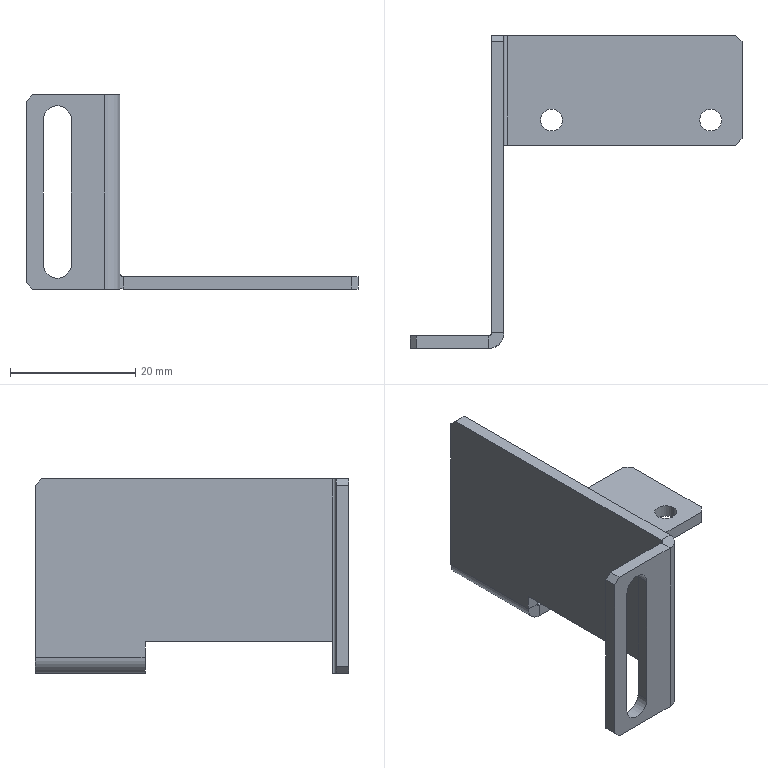Part | STEP file | 11-GX-ZB-04-006-A11 | 1 solid | 39 faces | box 53 x 50 x 31 mm | volume 4591 mm3 | plane 29 | cylinder 10 | commonest cylinder face diameters 3.5 x4 1 x2 4.5 x2 5 x2
STEP:
#1=CARTESIAN_POINT('',(34.75,-13.5,0.));
#2=VERTEX_POINT('',#1);
#3=CARTESIAN_POINT('',(31.25,-13.5,0.));
#4=VERTEX_POINT('',#3);
#5=CARTESIAN_POINT('',(33.,-13.5,0.));
#6=DIRECTION('',(0.,0.,-1.));
#7=DIRECTION('',(-1.,0.,0.));
#8=AXIS2_PLACEMENT_3D('',#5,#6,#7);
#9=CIRCLE('',#8,1.75);
#10=EDGE_CURVE('',#2,#4,#9,.T.);
#11=ORIENTED_EDGE('',*,*,#10,.T.);
#12=CARTESIAN_POINT('',(31.25,-13.5,2.));
#13=VERTEX_POINT('',#12);
#14=CARTESIAN_POINT('',(31.25,-13.5,-8.));
#15=DIRECTION('',(0.,0.,1.));
#16=VECTOR('',#15,1000.);
#17=LINE('',#14,#16);
#18=EDGE_CURVE('',#4,#13,#17,.T.);
#19=ORIENTED_EDGE('',*,*,#18,.T.);
#20=CARTESIAN_POINT('',(34.75,-13.5,2.));
#21=VERTEX_POINT('',#20);
#22=CARTESIAN_POINT('',(33.,-13.5,2.));
#23=DIRECTION('',(0.,0.,1.));
#24=DIRECTION('',(1.,0.,0.));
#25=AXIS2_PLACEMENT_3D('',#22,#23,#24);
#26=CIRCLE('',#25,1.75);
#27=EDGE_CURVE('',#13,#21,#26,.T.);
#28=ORIENTED_EDGE('',*,*,#27,.T.);
#29=CARTESIAN_POINT('',(34.75,-13.5,-8.));
#30=DIRECTION('',(0.,0.,1.));
#31=VECTOR('',#30,1000.);
#32=LINE('',#29,#31);
#33=EDGE_CURVE('',#2,#21,#32,.T.);
#34=ORIENTED_EDGE('',*,*,#33,.F.);
#35=EDGE_LOOP('',(#11,#19,#28,#34));
#36=FACE_OUTER_BOUND('',#35,.T.);
#37=CARTESIAN_POINT('',(33.,-13.5,-8.));
#38=DIRECTION('',(0.,0.,1.));
#39=DIRECTION('',(1.,0.,0.));
#40=AXIS2_PLACEMENT_3D('',#37,#38,#39);
#41=CYLINDRICAL_SURFACE('',#40,1.75);
#42=ADVANCED_FACE('',(#36),#41,.F.);
#43=CARTESIAN_POINT('',(9.35,-13.5,0.));
#44=VERTEX_POINT('',#43);
#45=CARTESIAN_POINT('',(5.85,-13.5,0.));
#46=VERTEX_POINT('',#45);
#47=CARTESIAN_POINT('',(7.6,-13.5,0.));
#48=DIRECTION('',(0.,0.,-1.));
#49=DIRECTION('',(-1.,0.,0.));
#50=AXIS2_PLACEMENT_3D('',#47,#48,#49);
#51=CIRCLE('',#50,1.75);
#52=EDGE_CURVE('',#44,#46,#51,.T.);
#53=ORIENTED_EDGE('',*,*,#52,.T.);
#54=CARTESIAN_POINT('',(5.85,-13.5,2.));
#55=VERTEX_POINT('',#54);
#56=CARTESIAN_POINT('',(5.85,-13.5,-8.));
#57=DIRECTION('',(0.,0.,1.));
#58=VECTOR('',#57,1000.);
#59=LINE('',#56,#58);
#60=EDGE_CURVE('',#46,#55,#59,.T.);
#61=ORIENTED_EDGE('',*,*,#60,.T.);
#62=CARTESIAN_POINT('',(9.35,-13.5,2.));
#63=VERTEX_POINT('',#62);
#64=CARTESIAN_POINT('',(7.6,-13.5,2.));
#65=DIRECTION('',(0.,0.,1.));
#66=DIRECTION('',(1.,0.,0.));
#67=AXIS2_PLACEMENT_3D('',#64,#65,#66);
#68=CIRCLE('',#67,1.75);
#69=EDGE_CURVE('',#55,#63,#68,.T.);
#70=ORIENTED_EDGE('',*,*,#69,.T.);
#71=CARTESIAN_POINT('',(9.35,-13.5,-8.));
#72=DIRECTION('',(0.,0.,1.));
#73=VECTOR('',#72,1000.);
#74=LINE('',#71,#73);
#75=EDGE_CURVE('',#44,#63,#74,.T.);
#76=ORIENTED_EDGE('',*,*,#75,.F.);
#77=EDGE_LOOP('',(#53,#61,#70,#76));
#78=FACE_OUTER_BOUND('',#77,.T.);
#79=CARTESIAN_POINT('',(7.6,-13.5,-8.));
#80=DIRECTION('',(0.,0.,1.));
#81=DIRECTION('',(1.,0.,0.));
#82=AXIS2_PLACEMENT_3D('',#79,#80,#81);
#83=CYLINDRICAL_SURFACE('',#82,1.75);
#84=ADVANCED_FACE('',(#78),#83,.F.);
#85=CARTESIAN_POINT('',(-2.,-1.,31.));
#86=VERTEX_POINT('',#85);
#87=CARTESIAN_POINT('',(-2.,-47.5,31.));
#88=VERTEX_POINT('',#87);
#89=CARTESIAN_POINT('',(-2.,0.,31.));
#90=DIRECTION('',(0.,-1.,0.));
#91=VECTOR('',#90,1000.);
#92=LINE('',#89,#91);
#93=EDGE_CURVE('',#86,#88,#92,.T.);
#94=ORIENTED_EDGE('',*,*,#93,.F.);
#95=CARTESIAN_POINT('',(-2.,0.,30.));
#96=VERTEX_POINT('',#95);
#97=CARTESIAN_POINT('',(-2.,0.,30.));
#98=DIRECTION('',(0.,0.7071,-0.7071));
#99=VECTOR('',#98,1000.);
#100=LINE('',#97,#99);
#101=EDGE_CURVE('',#86,#96,#100,.T.);
#102=ORIENTED_EDGE('',*,*,#101,.T.);
#103=CARTESIAN_POINT('',(-2.,0.,2.5));
#104=VERTEX_POINT('',#103);
#105=CARTESIAN_POINT('',(-2.,0.,31.));
#106=DIRECTION('',(0.,0.,-1.));
#107=VECTOR('',#106,1000.);
#108=LINE('',#105,#107);
#109=EDGE_CURVE('',#96,#104,#108,.T.);
#110=ORIENTED_EDGE('',*,*,#109,.T.);
#111=CARTESIAN_POINT('',(-2.,-17.5,2.5));
#112=VERTEX_POINT('',#111);
#113=CARTESIAN_POINT('',(-2.,0.,2.5));
#114=DIRECTION('',(0.,-1.,0.));
#115=VECTOR('',#114,1000.);
#116=LINE('',#113,#115);
#117=EDGE_CURVE('',#104,#112,#116,.T.);
#118=ORIENTED_EDGE('',*,*,#117,.T.);
#119=CARTESIAN_POINT('',(-2.,-17.5,5.));
#120=VERTEX_POINT('',#119);
#121=CARTESIAN_POINT('',(-2.,-17.5,31.));
#122=DIRECTION('',(0.,0.,1.));
#123=VECTOR('',#122,1000.);
#124=LINE('',#121,#123);
#125=EDGE_CURVE('',#112,#120,#124,.T.);
#126=ORIENTED_EDGE('',*,*,#125,.T.);
#127=CARTESIAN_POINT('',(-2.,-47.5,5.));
#128=VERTEX_POINT('',#127);
#129=CARTESIAN_POINT('',(-2.,0.,5.));
#130=DIRECTION('',(0.,-1.,0.));
#131=VECTOR('',#130,1000.);
#132=LINE('',#129,#131);
#133=EDGE_CURVE('',#120,#128,#132,.T.);
#134=ORIENTED_EDGE('',*,*,#133,.T.);
#135=CARTESIAN_POINT('',(-2.,-47.5,31.));
#136=DIRECTION('',(0.,0.,-1.));
#137=VECTOR('',#136,1000.);
#138=LINE('',#135,#137);
#139=EDGE_CURVE('',#88,#128,#138,.T.);
#140=ORIENTED_EDGE('',*,*,#139,.F.);
#141=EDGE_LOOP('',(#94,#102,#110,#118,#126,#134,#140));
#142=FACE_OUTER_BOUND('',#141,.T.);
#143=CARTESIAN_POINT('',(-2.,0.,31.));
#144=DIRECTION('',(1.,0.,0.));
#145=DIRECTION('',(0.,1.,0.));
#146=AXIS2_PLACEMENT_3D('',#143,#144,#145);
#147=PLANE('',#146);
#148=ADVANCED_FACE('',(#142),#147,.F.);
#149=CARTESIAN_POINT('',(0.,0.,30.));
#150=VERTEX_POINT('',#149);
#151=CARTESIAN_POINT('',(0.,0.,2.5));
#152=VERTEX_POINT('',#151);
#153=CARTESIAN_POINT('',(0.,0.,31.));
#154=DIRECTION('',(0.,0.,-1.));
#155=VECTOR('',#154,1000.);
#156=LINE('',#153,#155);
#157=EDGE_CURVE('',#150,#152,#156,.T.);
#158=ORIENTED_EDGE('',*,*,#157,.F.);
#159=CARTESIAN_POINT('',(0.,-1.,31.));
#160=VERTEX_POINT('',#159);
#161=CARTESIAN_POINT('',(0.,-0.5,30.5));
#162=DIRECTION('',(0.,-0.7071,0.7071));
#163=VECTOR('',#162,1000.);
#164=LINE('',#161,#163);
#165=EDGE_CURVE('',#150,#160,#164,.T.);
#166=ORIENTED_EDGE('',*,*,#165,.T.);
#167=CARTESIAN_POINT('',(0.,-47.5,31.));
#168=VERTEX_POINT('',#167);
#169=CARTESIAN_POINT('',(0.,0.,31.));
#170=DIRECTION('',(0.,-1.,0.));
#171=VECTOR('',#170,1000.);
#172=LINE('',#169,#171);
#173=EDGE_CURVE('',#160,#168,#172,.T.);
#174=ORIENTED_EDGE('',*,*,#173,.T.);
#175=CARTESIAN_POINT('',(0.,-47.5,5.));
#176=VERTEX_POINT('',#175);
#177=CARTESIAN_POINT('',(0.,-47.5,31.));
#178=DIRECTION('',(0.,0.,-1.));
#179=VECTOR('',#178,1000.);
#180=LINE('',#177,#179);
#181=EDGE_CURVE('',#168,#176,#180,.T.);
#182=ORIENTED_EDGE('',*,*,#181,.T.);
#183=CARTESIAN_POINT('',(0.,-17.5,5.));
#184=VERTEX_POINT('',#183);
#185=CARTESIAN_POINT('',(0.,0.,5.));
#186=DIRECTION('',(0.,-1.,0.));
#187=VECTOR('',#186,1000.);
#188=LINE('',#185,#187);
#189=EDGE_CURVE('',#184,#176,#188,.T.);
#190=ORIENTED_EDGE('',*,*,#189,.F.);
#191=CARTESIAN_POINT('',(0.,-17.5,2.5));
#192=VERTEX_POINT('',#191);
#193=CARTESIAN_POINT('',(0.,-17.5,31.));
#194=DIRECTION('',(0.,0.,1.));
#195=VECTOR('',#194,1000.);
#196=LINE('',#193,#195);
#197=EDGE_CURVE('',#192,#184,#196,.T.);
#198=ORIENTED_EDGE('',*,*,#197,.F.);
#199=CARTESIAN_POINT('',(0.,0.,2.5));
#200=DIRECTION('',(0.,-1.,0.));
#201=VECTOR('',#200,1000.);
#202=LINE('',#199,#201);
#203=EDGE_CURVE('',#152,#192,#202,.T.);
#204=ORIENTED_EDGE('',*,*,#203,.F.);
#205=EDGE_LOOP('',(#158,#166,#174,#182,#190,#198,#204));
#206=FACE_OUTER_BOUND('',#205,.T.);
#207=CARTESIAN_POINT('',(0.,0.,31.));
#208=DIRECTION('',(1.,0.,0.));
#209=DIRECTION('',(0.,1.,0.));
#210=AXIS2_PLACEMENT_3D('',#207,#208,#209);
#211=PLANE('',#210);
#212=ADVANCED_FACE('',(#206),#211,.T.);
#213=CARTESIAN_POINT('',(0.5,-17.5,0.));
#214=VERTEX_POINT('',#213);
#215=CARTESIAN_POINT('',(0.5,0.,0.));
#216=VERTEX_POINT('',#215);
#217=CARTESIAN_POINT('',(0.5,0.,0.));
#218=DIRECTION('',(0.,1.,0.));
#219=VECTOR('',#218,1000.);
#220=LINE('',#217,#219);
#221=EDGE_CURVE('',#214,#216,#220,.T.);
#222=ORIENTED_EDGE('',*,*,#221,.F.);
#223=CARTESIAN_POINT('',(0.5,-17.5,2.5));
#224=DIRECTION('',(0.,-1.,0.));
#225=DIRECTION('',(-1.,0.,0.));
#226=AXIS2_PLACEMENT_3D('',#223,#224,#225);
#227=CIRCLE('',#226,2.5);
#228=EDGE_CURVE('',#112,#214,#227,.T.);
#229=ORIENTED_EDGE('',*,*,#228,.F.);
#230=ORIENTED_EDGE('',*,*,#117,.F.);
#231=CARTESIAN_POINT('',(0.5,0.,2.5));
#232=DIRECTION('',(0.,1.,0.));
#233=DIRECTION('',(0.,0.,1.));
#234=AXIS2_PLACEMENT_3D('',#231,#232,#233);
#235=CIRCLE('',#234,2.5);
#236=EDGE_CURVE('',#216,#104,#235,.T.);
#237=ORIENTED_EDGE('',*,*,#236,.F.);
#238=EDGE_LOOP('',(#222,#229,#230,#237));
#239=FACE_OUTER_BOUND('',#238,.T.);
#240=CARTESIAN_POINT('',(0.5,0.,2.5));
#241=DIRECTION('',(0.,1.,0.));
#242=DIRECTION('',(0.,0.,-1.));
#243=AXIS2_PLACEMENT_3D('',#240,#241,#242);
#244=CYLINDRICAL_SURFACE('',#243,2.5);
#245=ADVANCED_FACE('',(#239),#244,.T.);
#246=CARTESIAN_POINT('',(0.5,-17.5,2.));
#247=VERTEX_POINT('',#246);
#248=CARTESIAN_POINT('',(0.5,-17.5,2.5));
#249=DIRECTION('',(0.,-1.,0.));
#250=DIRECTION('',(0.,0.,1.));
#251=AXIS2_PLACEMENT_3D('',#248,#249,#250);
#252=CIRCLE('',#251,0.5);
#253=EDGE_CURVE('',#192,#247,#252,.T.);
#254=ORIENTED_EDGE('',*,*,#253,.T.);
#255=CARTESIAN_POINT('',(0.5,0.,2.));
#256=VERTEX_POINT('',#255);
#257=CARTESIAN_POINT('',(0.5,-47.5,2.));
#258=DIRECTION('',(0.,1.,0.));
#259=VECTOR('',#258,1000.);
#260=LINE('',#257,#259);
#261=EDGE_CURVE('',#247,#256,#260,.T.);
#262=ORIENTED_EDGE('',*,*,#261,.T.);
#263=CARTESIAN_POINT('',(0.5,0.,2.5));
#264=DIRECTION('',(0.,1.,0.));
#265=DIRECTION('',(0.,0.,1.));
#266=AXIS2_PLACEMENT_3D('',#263,#264,#265);
#267=CIRCLE('',#266,0.5);
#268=EDGE_CURVE('',#256,#152,#267,.T.);
#269=ORIENTED_EDGE('',*,*,#268,.T.);
#270=ORIENTED_EDGE('',*,*,#203,.T.);
#271=EDGE_LOOP('',(#254,#262,#269,#270));
#272=FACE_OUTER_BOUND('',#271,.T.);
#273=CARTESIAN_POINT('',(0.5,0.,2.5));
#274=DIRECTION('',(0.,1.,0.));
#275=DIRECTION('',(0.,0.,-1.));
#276=AXIS2_PLACEMENT_3D('',#273,#274,#275);
#277=CYLINDRICAL_SURFACE('',#276,0.5);
#278=ADVANCED_FACE('',(#272),#277,.F.);
#279=ORIENTED_EDGE('',*,*,#10,.F.);
#280=CARTESIAN_POINT('',(33.,-13.5,0.));
#281=DIRECTION('',(0.,0.,-1.));
#282=DIRECTION('',(-1.,0.,0.));
#283=AXIS2_PLACEMENT_3D('',#280,#281,#282);
#284=CIRCLE('',#283,1.75);
#285=EDGE_CURVE('',#4,#2,#284,.T.);
#286=ORIENTED_EDGE('',*,*,#285,.F.);
#287=EDGE_LOOP('',(#279,#286));
#288=FACE_BOUND('',#287,.T.);
#289=ORIENTED_EDGE('',*,*,#52,.F.);
#290=CARTESIAN_POINT('',(7.6,-13.5,0.));
#291=DIRECTION('',(0.,0.,-1.));
#292=DIRECTION('',(-1.,0.,0.));
#293=AXIS2_PLACEMENT_3D('',#290,#291,#292);
#294=CIRCLE('',#293,1.75);
#295=EDGE_CURVE('',#46,#44,#294,.T.);
#296=ORIENTED_EDGE('',*,*,#295,.F.);
#297=EDGE_LOOP('',(#289,#296));
#298=FACE_BOUND('',#297,.T.);
#299=CARTESIAN_POINT('',(37.,0.,0.));
#300=VERTEX_POINT('',#299);
#301=CARTESIAN_POINT('',(0.,0.,0.));
#302=DIRECTION('',(-1.,0.,0.));
#303=VECTOR('',#302,1000.);
#304=LINE('',#301,#303);
#305=EDGE_CURVE('',#300,#216,#304,.T.);
#306=ORIENTED_EDGE('',*,*,#305,.F.);
#307=CARTESIAN_POINT('',(38.,-1.,0.));
#308=VERTEX_POINT('',#307);
#309=CARTESIAN_POINT('',(18.5,18.5,0.));
#310=DIRECTION('',(0.7071,-0.7071,0.));
#311=VECTOR('',#310,1000.);
#312=LINE('',#309,#311);
#313=EDGE_CURVE('',#300,#308,#312,.T.);
#314=ORIENTED_EDGE('',*,*,#313,.T.);
#315=CARTESIAN_POINT('',(38.,-16.5,0.));
#316=VERTEX_POINT('',#315);
#317=CARTESIAN_POINT('',(38.,0.,0.));
#318=DIRECTION('',(0.,1.,0.));
#319=VECTOR('',#318,1000.);
#320=LINE('',#317,#319);
#321=EDGE_CURVE('',#316,#308,#320,.T.);
#322=ORIENTED_EDGE('',*,*,#321,.F.);
#323=CARTESIAN_POINT('',(37.,-17.5,0.));
#324=VERTEX_POINT('',#323);
#325=CARTESIAN_POINT('',(27.25,-27.25,0.));
#326=DIRECTION('',(-0.7071,-0.7071,0.));
#327=VECTOR('',#326,1000.);
#328=LINE('',#325,#327);
#329=EDGE_CURVE('',#316,#324,#328,.T.);
#330=ORIENTED_EDGE('',*,*,#329,.T.);
#331=CARTESIAN_POINT('',(0.,-17.5,0.));
#332=DIRECTION('',(1.,0.,0.));
#333=VECTOR('',#332,1000.);
#334=LINE('',#331,#333);
#335=EDGE_CURVE('',#214,#324,#334,.T.);
#336=ORIENTED_EDGE('',*,*,#335,.F.);
#337=ORIENTED_EDGE('',*,*,#221,.T.);
#338=EDGE_LOOP('',(#306,#314,#322,#330,#336,#337));
#339=FACE_OUTER_BOUND('',#338,.T.);
#340=CARTESIAN_POINT('',(0.,0.,0.));
#341=DIRECTION('',(0.,0.,-1.));
#342=DIRECTION('',(-1.,0.,0.));
#343=AXIS2_PLACEMENT_3D('',#340,#341,#342);
#344=PLANE('',#343);
#345=ADVANCED_FACE('',(#288,#298,#339),#344,.T.);
#346=CARTESIAN_POINT('',(33.,-13.5,2.));
#347=DIRECTION('',(0.,0.,1.));
#348=DIRECTION('',(1.,0.,0.));
#349=AXIS2_PLACEMENT_3D('',#346,#347,#348);
#350=CIRCLE('',#349,1.75);
#351=EDGE_CURVE('',#21,#13,#350,.T.);
#352=ORIENTED_EDGE('',*,*,#351,.F.);
#353=ORIENTED_EDGE('',*,*,#27,.F.);
#354=EDGE_LOOP('',(#352,#353));
#355=FACE_BOUND('',#354,.T.);
#356=CARTESIAN_POINT('',(7.6,-13.5,2.));
#357=DIRECTION('',(0.,0.,1.));
#358=DIRECTION('',(1.,0.,0.));
#359=AXIS2_PLACEMENT_3D('',#356,#357,#358);
#360=CIRCLE('',#359,1.75);
#361=EDGE_CURVE('',#63,#55,#360,.T.);
#362=ORIENTED_EDGE('',*,*,#361,.F.);
#363=ORIENTED_EDGE('',*,*,#69,.F.);
#364=EDGE_LOOP('',(#362,#363));
#365=FACE_BOUND('',#364,.T.);
#366=CARTESIAN_POINT('',(38.,-16.5,2.));
#367=VERTEX_POINT('',#366);
#368=CARTESIAN_POINT('',(38.,-1.,2.));
#369=VERTEX_POINT('',#368);
#370=CARTESIAN_POINT('',(38.,0.,2.));
#371=DIRECTION('',(0.,1.,0.));
#372=VECTOR('',#371,1000.);
#373=LINE('',#370,#372);
#374=EDGE_CURVE('',#367,#369,#373,.T.);
#375=ORIENTED_EDGE('',*,*,#374,.T.);
#376=CARTESIAN_POINT('',(37.,0.,2.));
#377=VERTEX_POINT('',#376);
#378=CARTESIAN_POINT('',(38.,-1.,2.));
#379=DIRECTION('',(-0.7071,0.7071,0.));
#380=VECTOR('',#379,1000.);
#381=LINE('',#378,#380);
#382=EDGE_CURVE('',#369,#377,#381,.T.);
#383=ORIENTED_EDGE('',*,*,#382,.T.);
#384=CARTESIAN_POINT('',(0.,0.,2.));
#385=DIRECTION('',(-1.,0.,0.));
#386=VECTOR('',#385,1000.);
#387=LINE('',#384,#386);
#388=EDGE_CURVE('',#377,#256,#387,.T.);
#389=ORIENTED_EDGE('',*,*,#388,.T.);
#390=ORIENTED_EDGE('',*,*,#261,.F.);
#391=CARTESIAN_POINT('',(37.,-17.5,2.));
#392=VERTEX_POINT('',#391);
#393=CARTESIAN_POINT('',(0.,-17.5,2.));
#394=DIRECTION('',(1.,0.,0.));
#395=VECTOR('',#394,1000.);
#396=LINE('',#393,#395);
#397=EDGE_CURVE('',#247,#392,#396,.T.);
#398=ORIENTED_EDGE('',*,*,#397,.T.);
#399=CARTESIAN_POINT('',(38.,-16.5,2.));
#400=DIRECTION('',(0.7071,0.7071,0.));
#401=VECTOR('',#400,1000.);
#402=LINE('',#399,#401);
#403=EDGE_CURVE('',#392,#367,#402,.T.);
#404=ORIENTED_EDGE('',*,*,#403,.T.);
#405=EDGE_LOOP('',(#375,#383,#389,#390,#398,#404));
#406=FACE_OUTER_BOUND('',#405,.T.);
#407=CARTESIAN_POINT('',(0.,0.,2.));
#408=DIRECTION('',(0.,0.,-1.));
#409=DIRECTION('',(-1.,0.,0.));
#410=AXIS2_PLACEMENT_3D('',#407,#408,#409);
#411=PLANE('',#410);
#412=ADVANCED_FACE('',(#355,#365,#406),#411,.F.);
#413=ORIENTED_EDGE('',*,*,#321,.T.);
#414=CARTESIAN_POINT('',(38.,-1.,0.));
#415=DIRECTION('',(0.,0.,1.));
#416=VECTOR('',#415,1000.);
#417=LINE('',#414,#416);
#418=EDGE_CURVE('',#308,#369,#417,.T.);
#419=ORIENTED_EDGE('',*,*,#418,.T.);
#420=ORIENTED_EDGE('',*,*,#374,.F.);
#421=CARTESIAN_POINT('',(38.,-16.5,0.));
#422=DIRECTION('',(0.,0.,-1.));
#423=VECTOR('',#422,1000.);
#424=LINE('',#421,#423);
#425=EDGE_CURVE('',#367,#316,#424,.T.);
#426=ORIENTED_EDGE('',*,*,#425,.T.);
#427=EDGE_LOOP('',(#413,#419,#420,#426));
#428=FACE_OUTER_BOUND('',#427,.T.);
#429=CARTESIAN_POINT('',(38.,0.,0.));
#430=DIRECTION('',(1.,0.,0.));
#431=DIRECTION('',(0.,0.,-1.));
#432=AXIS2_PLACEMENT_3D('',#429,#430,#431);
#433=PLANE('',#432);
#434=ADVANCED_FACE('',(#428),#433,.T.);
#435=CARTESIAN_POINT('',(-2.,-47.5,2.5));
#436=VERTEX_POINT('',#435);
#437=CARTESIAN_POINT('',(-2.,-47.5,0.));
#438=VERTEX_POINT('',#437);
#439=CARTESIAN_POINT('',(-2.,-47.5,31.));
#440=DIRECTION('',(0.,0.,-1.));
#441=VECTOR('',#440,1000.);
#442=LINE('',#439,#441);
#443=EDGE_CURVE('',#436,#438,#442,.T.);
#444=ORIENTED_EDGE('',*,*,#443,.F.);
#445=CARTESIAN_POINT('',(0.,-47.5,0.05051));
#446=VERTEX_POINT('',#445);
#447=CARTESIAN_POINT('',(0.5,-47.5,2.5));
#448=DIRECTION('',(0.,-1.,0.));
#449=DIRECTION('',(0.,0.,1.));
#450=AXIS2_PLACEMENT_3D('',#447,#448,#449);
#451=CIRCLE('',#450,2.5);
#452=EDGE_CURVE('',#436,#446,#451,.T.);
#453=ORIENTED_EDGE('',*,*,#452,.T.);
#454=CARTESIAN_POINT('',(0.,-47.5,0.));
#455=VERTEX_POINT('',#454);
#456=CARTESIAN_POINT('',(0.,-47.5,2.5));
#457=DIRECTION('',(0.,0.,-1.));
#458=VECTOR('',#457,1000.);
#459=LINE('',#456,#458);
#460=EDGE_CURVE('',#446,#455,#459,.T.);
#461=ORIENTED_EDGE('',*,*,#460,.T.);
#462=CARTESIAN_POINT('',(-2.,-47.5,0.));
#463=DIRECTION('',(1.,0.,0.));
#464=VECTOR('',#463,1000.);
#465=LINE('',#462,#464);
#466=EDGE_CURVE('',#438,#455,#465,.T.);
#467=ORIENTED_EDGE('',*,*,#466,.F.);
#468=EDGE_LOOP('',(#444,#453,#461,#467));
#469=FACE_OUTER_BOUND('',#468,.T.);
#470=CARTESIAN_POINT('',(0.,-47.5,2.5));
#471=DIRECTION('',(0.,1.,0.));
#472=DIRECTION('',(-1.,0.,0.));
#473=AXIS2_PLACEMENT_3D('',#470,#471,#472);
#474=PLANE('',#473);
#475=ADVANCED_FACE('',(#469),#474,.T.);
#476=ORIENTED_EDGE('',*,*,#109,.F.);
#477=CARTESIAN_POINT('',(0.,0.,30.));
#478=DIRECTION('',(1.,0.,0.));
#479=VECTOR('',#478,1000.);
#480=LINE('',#477,#479);
#481=EDGE_CURVE('',#96,#150,#480,.T.);
#482=ORIENTED_EDGE('',*,*,#481,.T.);
#483=ORIENTED_EDGE('',*,*,#157,.T.);
#484=CARTESIAN_POINT('',(0.,0.,2.5));
#485=DIRECTION('',(-1.,0.,0.));
#486=VECTOR('',#485,1000.);
#487=LINE('',#484,#486);
#488=EDGE_CURVE('',#152,#104,#487,.T.);
#489=ORIENTED_EDGE('',*,*,#488,.T.);
#490=EDGE_LOOP('',(#476,#482,#483,#489));
#491=FACE_OUTER_BOUND('',#490,.T.);
#492=CARTESIAN_POINT('',(-2.,0.,31.));
#493=DIRECTION('',(0.,1.,0.));
#494=DIRECTION('',(-1.,0.,0.));
#495=AXIS2_PLACEMENT_3D('',#492,#493,#494);
#496=PLANE('',#495);
#497=ADVANCED_FACE('',(#491),#496,.T.);
#498=ORIENTED_EDGE('',*,*,#173,.F.);
#499=CARTESIAN_POINT('',(-2.,-1.,31.));
#500=DIRECTION('',(-1.,0.,0.));
#501=VECTOR('',#500,1000.);
#502=LINE('',#499,#501);
#503=EDGE_CURVE('',#160,#86,#502,.T.);
#504=ORIENTED_EDGE('',*,*,#503,.T.);
#505=ORIENTED_EDGE('',*,*,#93,.T.);
#506=CARTESIAN_POINT('',(-2.,-47.5,31.));
#507=DIRECTION('',(1.,0.,0.));
#508=VECTOR('',#507,1000.);
#509=LINE('',#506,#508);
#510=EDGE_CURVE('',#88,#168,#509,.T.);
#511=ORIENTED_EDGE('',*,*,#510,.T.);
#512=EDGE_LOOP('',(#498,#504,#505,#511));
#513=FACE_OUTER_BOUND('',#512,.T.);
#514=CARTESIAN_POINT('',(0.,0.,31.));
#515=DIRECTION('',(0.,0.,-1.));
#516=DIRECTION('',(-1.,0.,0.));
#517=AXIS2_PLACEMENT_3D('',#514,#515,#516);
#518=PLANE('',#517);
#519=ADVANCED_FACE('',(#513),#518,.F.);
#520=CARTESIAN_POINT('',(-2.5,-48.,0.));
#521=VERTEX_POINT('',#520);
#522=CARTESIAN_POINT('',(-2.5,-50.,0.));
#523=VERTEX_POINT('',#522);
#524=CARTESIAN_POINT('',(-2.5,-50.,0.));
#525=DIRECTION('',(0.,-1.,0.));
#526=VECTOR('',#525,1000.);
#527=LINE('',#524,#526);
#528=EDGE_CURVE('',#521,#523,#527,.T.);
#529=ORIENTED_EDGE('',*,*,#528,.F.);
#530=CARTESIAN_POINT('',(-2.5,-47.5,0.));
#531=DIRECTION('',(0.,0.,-1.));
#532=DIRECTION('',(1.,0.,0.));
#533=AXIS2_PLACEMENT_3D('',#530,#531,#532);
#534=CIRCLE('',#533,0.5);
#535=EDGE_CURVE('',#438,#521,#534,.T.);
#536=ORIENTED_EDGE('',*,*,#535,.F.);
#537=ORIENTED_EDGE('',*,*,#466,.T.);
#538=CARTESIAN_POINT('',(-2.5,-47.5,0.));
#539=DIRECTION('',(0.,0.,-1.));
#540=DIRECTION('',(1.,0.,0.));
#541=AXIS2_PLACEMENT_3D('',#538,#539,#540);
#542=CIRCLE('',#541,2.5);
#543=EDGE_CURVE('',#455,#523,#542,.T.);
#544=ORIENTED_EDGE('',*,*,#543,.T.);
#545=EDGE_LOOP('',(#529,#536,#537,#544));
#546=FACE_OUTER_BOUND('',#545,.T.);
#547=CARTESIAN_POINT('',(-2.5,-47.5,0.));
#548=DIRECTION('',(0.,0.,-1.));
#549=DIRECTION('',(-1.,0.,0.));
#550=AXIS2_PLACEMENT_3D('',#547,#548,#549);
#551=PLANE('',#550);
#552=ADVANCED_FACE('',(#546),#551,.T.);
#553=CARTESIAN_POINT('',(-2.5,-48.,31.));
#554=VERTEX_POINT('',#553);
#555=CARTESIAN_POINT('',(-2.5,-47.5,31.));
#556=DIRECTION('',(0.,0.,1.));
#557=DIRECTION('',(1.,0.,0.));
#558=AXIS2_PLACEMENT_3D('',#555,#556,#557);
#559=CIRCLE('',#558,0.5);
#560=EDGE_CURVE('',#554,#88,#559,.T.);
#561=ORIENTED_EDGE('',*,*,#560,.F.);
#562=CARTESIAN_POINT('',(-2.5,-50.,31.));
#563=VERTEX_POINT('',#562);
#564=CARTESIAN_POINT('',(-2.5,-48.,31.));
#565=DIRECTION('',(0.,-1.,0.));
#566=VECTOR('',#565,1000.);
#567=LINE('',#564,#566);
#568=EDGE_CURVE('',#554,#563,#567,.T.);
#569=ORIENTED_EDGE('',*,*,#568,.T.);
#570=CARTESIAN_POINT('',(-2.5,-47.5,31.));
#571=DIRECTION('',(0.,0.,1.));
#572=DIRECTION('',(1.,0.,0.));
#573=AXIS2_PLACEMENT_3D('',#570,#571,#572);
#574=CIRCLE('',#573,2.5);
#575=EDGE_CURVE('',#563,#168,#574,.T.);
#576=ORIENTED_EDGE('',*,*,#575,.T.);
#577=ORIENTED_EDGE('',*,*,#510,.F.);
#578=EDGE_LOOP('',(#561,#569,#576,#577));
#579=FACE_OUTER_BOUND('',#578,.T.);
#580=CARTESIAN_POINT('',(-2.5,-47.5,31.));
#581=DIRECTION('',(0.,0.,-1.));
#582=DIRECTION('',(-1.,0.,0.));
#583=AXIS2_PLACEMENT_3D('',#580,#581,#582);
#584=PLANE('',#583);
#585=ADVANCED_FACE('',(#579),#584,.F.);
#586=ORIENTED_EDGE('',*,*,#181,.F.);
#587=ORIENTED_EDGE('',*,*,#575,.F.);
#588=CARTESIAN_POINT('',(-2.5,-50.,0.));
#589=DIRECTION('',(0.,0.,-1.));
#590=VECTOR('',#589,1000.);
#591=LINE('',#588,#590);
#592=EDGE_CURVE('',#563,#523,#591,.T.);
#593=ORIENTED_EDGE('',*,*,#592,.T.);
#594=ORIENTED_EDGE('',*,*,#543,.F.);
#595=ORIENTED_EDGE('',*,*,#460,.F.);
#596=CARTESIAN_POINT('',(0.,-47.5,2.5));
#597=DIRECTION('',(0.,0.,-1.));
#598=VECTOR('',#597,1000.);
#599=LINE('',#596,#598);
#600=EDGE_CURVE('',#176,#446,#599,.T.);
#601=ORIENTED_EDGE('',*,*,#600,.F.);
#602=EDGE_LOOP('',(#586,#587,#593,#594,#595,#601));
#603=FACE_OUTER_BOUND('',#602,.T.);
#604=CARTESIAN_POINT('',(-2.5,-47.5,31.));
#605=DIRECTION('',(0.,0.,1.));
#606=DIRECTION('',(0.,-1.,0.));
#607=AXIS2_PLACEMENT_3D('',#604,#605,#606);
#608=CYLINDRICAL_SURFACE('',#607,2.5);
#609=ADVANCED_FACE('',(#603),#608,.T.);
#610=ORIENTED_EDGE('',*,*,#139,.T.);
#611=CARTESIAN_POINT('',(-2.,-47.5,31.));
#612=DIRECTION('',(0.,0.,-1.));
#613=VECTOR('',#612,1000.);
#614=LINE('',#611,#613);
#615=EDGE_CURVE('',#128,#436,#614,.T.);
#616=ORIENTED_EDGE('',*,*,#615,.T.);
#617=ORIENTED_EDGE('',*,*,#443,.T.);
#618=ORIENTED_EDGE('',*,*,#535,.T.);
#619=CARTESIAN_POINT('',(-2.5,-48.,0.));
#620=DIRECTION('',(0.,0.,1.));
#621=VECTOR('',#620,1000.);
#622=LINE('',#619,#621);
#623=EDGE_CURVE('',#521,#554,#622,.T.);
#624=ORIENTED_EDGE('',*,*,#623,.T.);
#625=ORIENTED_EDGE('',*,*,#560,.T.);
#626=EDGE_LOOP('',(#610,#616,#617,#618,#624,#625));
#627=FACE_OUTER_BOUND('',#626,.T.);
#628=CARTESIAN_POINT('',(-2.5,-47.5,31.));
#629=DIRECTION('',(0.,0.,1.));
#630=DIRECTION('',(0.,-1.,0.));
#631=AXIS2_PLACEMENT_3D('',#628,#629,#630);
#632=CYLINDRICAL_SURFACE('',#631,0.5);
#633=ADVANCED_FACE('',(#627),#632,.F.);
#634=CARTESIAN_POINT('',(-14.,-48.,31.));
#635=VERTEX_POINT('',#634);
#636=CARTESIAN_POINT('',(-15.,-48.,31.));
#637=DIRECTION('',(-1.,0.,0.));
#638=VECTOR('',#637,1000.);
#639=LINE('',#636,#638);
#640=EDGE_CURVE('',#554,#635,#639,.T.);
#641=ORIENTED_EDGE('',*,*,#640,.T.);
#642=CARTESIAN_POINT('',(-14.,-50.,31.));
#643=VERTEX_POINT('',#642);
#644=CARTESIAN_POINT('',(-14.,-50.,31.));
#645=DIRECTION('',(0.,-1.,0.));
#646=VECTOR('',#645,1000.);
#647=LINE('',#644,#646);
#648=EDGE_CURVE('',#635,#643,#647,.T.);
#649=ORIENTED_EDGE('',*,*,#648,.T.);
#650=CARTESIAN_POINT('',(0.,-50.,31.));
#651=DIRECTION('',(-1.,0.,0.));
#652=VECTOR('',#651,1000.);
#653=LINE('',#650,#652);
#654=EDGE_CURVE('',#563,#643,#653,.T.);
#655=ORIENTED_EDGE('',*,*,#654,.F.);
#656=ORIENTED_EDGE('',*,*,#568,.F.);
#657=EDGE_LOOP('',(#641,#649,#655,#656));
#658=FACE_OUTER_BOUND('',#657,.T.);
#659=CARTESIAN_POINT('',(-15.,-50.,31.));
#660=DIRECTION('',(0.,0.,-1.));
#661=DIRECTION('',(-1.,0.,0.));
#662=AXIS2_PLACEMENT_3D('',#659,#660,#661);
#663=PLANE('',#662);
#664=ADVANCED_FACE('',(#658),#663,.F.);
#665=CARTESIAN_POINT('',(-14.,-50.,0.));
#666=VERTEX_POINT('',#665);
#667=CARTESIAN_POINT('',(0.,-50.,0.));
#668=DIRECTION('',(1.,0.,0.));
#669=VECTOR('',#668,1000.);
#670=LINE('',#667,#669);
#671=EDGE_CURVE('',#666,#523,#670,.T.);
#672=ORIENTED_EDGE('',*,*,#671,.F.);
#673=CARTESIAN_POINT('',(-14.,-48.,0.));
#674=VERTEX_POINT('',#673);
#675=CARTESIAN_POINT('',(-14.,-50.,0.));
#676=DIRECTION('',(0.,1.,0.));
#677=VECTOR('',#676,1000.);
#678=LINE('',#675,#677);
#679=EDGE_CURVE('',#666,#674,#678,.T.);
#680=ORIENTED_EDGE('',*,*,#679,.T.);
#681=CARTESIAN_POINT('',(-2.,-48.,0.));
#682=DIRECTION('',(1.,0.,0.));
#683=VECTOR('',#682,1000.);
#684=LINE('',#681,#683);
#685=EDGE_CURVE('',#674,#521,#684,.T.);
#686=ORIENTED_EDGE('',*,*,#685,.T.);
#687=ORIENTED_EDGE('',*,*,#528,.T.);
#688=EDGE_LOOP('',(#672,#680,#686,#687));
#689=FACE_OUTER_BOUND('',#688,.T.);
#690=CARTESIAN_POINT('',(-2.,-50.,0.));
#691=DIRECTION('',(0.,0.,1.));
#692=DIRECTION('',(1.,0.,0.));
#693=AXIS2_PLACEMENT_3D('',#690,#691,#692);
#694=PLANE('',#693);
#695=ADVANCED_FACE('',(#689),#694,.F.);
#696=CARTESIAN_POINT('',(-7.75,-50.,27.));
#697=VERTEX_POINT('',#696);
#698=CARTESIAN_POINT('',(-7.75,-50.,4.));
#699=VERTEX_POINT('',#698);
#700=CARTESIAN_POINT('',(-7.75,-50.,0.));
#701=DIRECTION('',(0.,0.,-1.));
#702=VECTOR('',#701,1000.);
#703=LINE('',#700,#702);
#704=EDGE_CURVE('',#697,#699,#703,.T.);
#705=ORIENTED_EDGE('',*,*,#704,.T.);
#706=CARTESIAN_POINT('',(-12.25,-50.,4.));
#707=VERTEX_POINT('',#706);
#708=CARTESIAN_POINT('',(-10.,-50.,4.));
#709=DIRECTION('',(0.,1.,0.));
#710=DIRECTION('',(-1.,0.,0.));
#711=AXIS2_PLACEMENT_3D('',#708,#709,#710);
#712=CIRCLE('',#711,2.25);
#713=EDGE_CURVE('',#699,#707,#712,.T.);
#714=ORIENTED_EDGE('',*,*,#713,.T.);
#715=CARTESIAN_POINT('',(-12.25,-50.,27.));
#716=VERTEX_POINT('',#715);
#717=CARTESIAN_POINT('',(-12.25,-50.,0.));
#718=DIRECTION('',(0.,0.,1.));
#719=VECTOR('',#718,1000.);
#720=LINE('',#717,#719);
#721=EDGE_CURVE('',#707,#716,#720,.T.);
#722=ORIENTED_EDGE('',*,*,#721,.T.);
#723=CARTESIAN_POINT('',(-10.,-50.,27.));
#724=DIRECTION('',(0.,1.,0.));
#725=DIRECTION('',(-1.,0.,0.));
#726=AXIS2_PLACEMENT_3D('',#723,#724,#725);
#727=CIRCLE('',#726,2.25);
#728=EDGE_CURVE('',#716,#697,#727,.T.);
#729=ORIENTED_EDGE('',*,*,#728,.T.);
#730=EDGE_LOOP('',(#705,#714,#722,#729));
#731=FACE_BOUND('',#730,.T.);
#732=CARTESIAN_POINT('',(-15.,-50.,30.));
#733=VERTEX_POINT('',#732);
#734=CARTESIAN_POINT('',(-15.,-50.,1.));
#735=VERTEX_POINT('',#734);
#736=CARTESIAN_POINT('',(-15.,-50.,0.));
#737=DIRECTION('',(0.,0.,-1.));
#738=VECTOR('',#737,1000.);
#739=LINE('',#736,#738);
#740=EDGE_CURVE('',#733,#735,#739,.T.);
#741=ORIENTED_EDGE('',*,*,#740,.T.);
#742=CARTESIAN_POINT('',(-14.,-50.,0.));
#743=DIRECTION('',(0.7071,0.,-0.7071));
#744=VECTOR('',#743,1000.);
#745=LINE('',#742,#744);
#746=EDGE_CURVE('',#735,#666,#745,.T.);
#747=ORIENTED_EDGE('',*,*,#746,.T.);
#748=ORIENTED_EDGE('',*,*,#671,.T.);
#749=ORIENTED_EDGE('',*,*,#592,.F.);
#750=ORIENTED_EDGE('',*,*,#654,.T.);
#751=CARTESIAN_POINT('',(-15.,-50.,30.));
#752=DIRECTION('',(-0.7071,0.,-0.7071));
#753=VECTOR('',#752,1000.);
#754=LINE('',#751,#753);
#755=EDGE_CURVE('',#643,#733,#754,.T.);
#756=ORIENTED_EDGE('',*,*,#755,.T.);
#757=EDGE_LOOP('',(#741,#747,#748,#749,#750,#756));
#758=FACE_OUTER_BOUND('',#757,.T.);
#759=CARTESIAN_POINT('',(0.,-50.,0.));
#760=DIRECTION('',(0.,1.,0.));
#761=DIRECTION('',(-1.,0.,0.));
#762=AXIS2_PLACEMENT_3D('',#759,#760,#761);
#763=PLANE('',#762);
#764=ADVANCED_FACE('',(#731,#758),#763,.F.);
#765=CARTESIAN_POINT('',(-7.75,-48.,4.));
#766=VERTEX_POINT('',#765);
#767=CARTESIAN_POINT('',(-12.25,-48.,4.));
#768=VERTEX_POINT('',#767);
#769=CARTESIAN_POINT('',(-10.,-48.,4.));
#770=DIRECTION('',(0.,1.,0.));
#771=DIRECTION('',(-1.,0.,0.));
#772=AXIS2_PLACEMENT_3D('',#769,#770,#771);
#773=CIRCLE('',#772,2.25);
#774=EDGE_CURVE('',#766,#768,#773,.T.);
#775=ORIENTED_EDGE('',*,*,#774,.F.);
#776=CARTESIAN_POINT('',(-7.75,-48.,27.));
#777=VERTEX_POINT('',#776);
#778=CARTESIAN_POINT('',(-7.75,-48.,4.));
#779=DIRECTION('',(0.,0.,-1.));
#780=VECTOR('',#779,1000.);
#781=LINE('',#778,#780);
#782=EDGE_CURVE('',#777,#766,#781,.T.);
#783=ORIENTED_EDGE('',*,*,#782,.F.);
#784=CARTESIAN_POINT('',(-12.25,-48.,27.));
#785=VERTEX_POINT('',#784);
#786=CARTESIAN_POINT('',(-10.,-48.,27.));
#787=DIRECTION('',(0.,1.,0.));
#788=DIRECTION('',(-1.,0.,0.));
#789=AXIS2_PLACEMENT_3D('',#786,#787,#788);
#790=CIRCLE('',#789,2.25);
#791=EDGE_CURVE('',#785,#777,#790,.T.);
#792=ORIENTED_EDGE('',*,*,#791,.F.);
#793=CARTESIAN_POINT('',(-12.25,-48.,4.));
#794=DIRECTION('',(0.,0.,1.));
#795=VECTOR('',#794,1000.);
#796=LINE('',#793,#795);
#797=EDGE_CURVE('',#768,#785,#796,.T.);
#798=ORIENTED_EDGE('',*,*,#797,.F.);
#799=EDGE_LOOP('',(#775,#783,#792,#798));
#800=FACE_BOUND('',#799,.T.);
#801=ORIENTED_EDGE('',*,*,#685,.F.);
#802=CARTESIAN_POINT('',(-15.,-48.,1.));
#803=VERTEX_POINT('',#802);
#804=CARTESIAN_POINT('',(-7.,-48.,-7.));
#805=DIRECTION('',(-0.7071,0.,0.7071));
#806=VECTOR('',#805,1000.);
#807=LINE('',#804,#806);
#808=EDGE_CURVE('',#674,#803,#807,.T.);
#809=ORIENTED_EDGE('',*,*,#808,.T.);
#810=CARTESIAN_POINT('',(-15.,-48.,30.));
#811=VERTEX_POINT('',#810);
#812=CARTESIAN_POINT('',(-15.,-48.,0.));
#813=DIRECTION('',(0.,0.,-1.));
#814=VECTOR('',#813,1000.);
#815=LINE('',#812,#814);
#816=EDGE_CURVE('',#811,#803,#815,.T.);
#817=ORIENTED_EDGE('',*,*,#816,.F.);
#818=CARTESIAN_POINT('',(-22.5,-48.,22.5));
#819=DIRECTION('',(0.7071,0.,0.7071));
#820=VECTOR('',#819,1000.);
#821=LINE('',#818,#820);
#822=EDGE_CURVE('',#811,#635,#821,.T.);
#823=ORIENTED_EDGE('',*,*,#822,.T.);
#824=ORIENTED_EDGE('',*,*,#640,.F.);
#825=ORIENTED_EDGE('',*,*,#623,.F.);
#826=EDGE_LOOP('',(#801,#809,#817,#823,#824,#825));
#827=FACE_OUTER_BOUND('',#826,.T.);
#828=CARTESIAN_POINT('',(0.,-48.,0.));
#829=DIRECTION('',(0.,1.,0.));
#830=DIRECTION('',(-1.,0.,0.));
#831=AXIS2_PLACEMENT_3D('',#828,#829,#830);
#832=PLANE('',#831);
#833=ADVANCED_FACE('',(#800,#827),#832,.T.);
#834=ORIENTED_EDGE('',*,*,#816,.T.);
#835=CARTESIAN_POINT('',(-15.,-50.,1.));
#836=DIRECTION('',(0.,-1.,0.));
#837=VECTOR('',#836,1000.);
#838=LINE('',#835,#837);
#839=EDGE_CURVE('',#803,#735,#838,.T.);
#840=ORIENTED_EDGE('',*,*,#839,.T.);
#841=ORIENTED_EDGE('',*,*,#740,.F.);
#842=CARTESIAN_POINT('',(-15.,-50.,30.));
#843=DIRECTION('',(0.,1.,0.));
#844=VECTOR('',#843,1000.);
#845=LINE('',#842,#844);
#846=EDGE_CURVE('',#733,#811,#845,.T.);
#847=ORIENTED_EDGE('',*,*,#846,.T.);
#848=EDGE_LOOP('',(#834,#840,#841,#847));
#849=FACE_OUTER_BOUND('',#848,.T.);
#850=CARTESIAN_POINT('',(-15.,-50.,0.));
#851=DIRECTION('',(1.,0.,0.));
#852=DIRECTION('',(0.,1.,0.));
#853=AXIS2_PLACEMENT_3D('',#850,#851,#852);
#854=PLANE('',#853);
#855=ADVANCED_FACE('',(#849),#854,.F.);
#856=CARTESIAN_POINT('',(-7.75,-58.,4.));
#857=DIRECTION('',(0.,1.,0.));
#858=VECTOR('',#857,1000.);
#859=LINE('',#856,#858);
#860=EDGE_CURVE('',#699,#766,#859,.T.);
#861=ORIENTED_EDGE('',*,*,#860,.T.);
#862=ORIENTED_EDGE('',*,*,#774,.T.);
#863=CARTESIAN_POINT('',(-12.25,-58.,4.));
#864=DIRECTION('',(0.,1.,0.));
#865=VECTOR('',#864,1000.);
#866=LINE('',#863,#865);
#867=EDGE_CURVE('',#707,#768,#866,.T.);
#868=ORIENTED_EDGE('',*,*,#867,.F.);
#869=ORIENTED_EDGE('',*,*,#713,.F.);
#870=EDGE_LOOP('',(#861,#862,#868,#869));
#871=FACE_OUTER_BOUND('',#870,.T.);
#872=CARTESIAN_POINT('',(-10.,-58.,4.));
#873=DIRECTION('',(0.,1.,0.));
#874=DIRECTION('',(-1.,0.,0.));
#875=AXIS2_PLACEMENT_3D('',#872,#873,#874);
#876=CYLINDRICAL_SURFACE('',#875,2.25);
#877=ADVANCED_FACE('',(#871),#876,.F.);
#878=CARTESIAN_POINT('',(-7.75,-58.,27.));
#879=DIRECTION('',(0.,1.,0.));
#880=VECTOR('',#879,1000.);
#881=LINE('',#878,#880);
#882=EDGE_CURVE('',#697,#777,#881,.T.);
#883=ORIENTED_EDGE('',*,*,#882,.T.);
#884=ORIENTED_EDGE('',*,*,#782,.T.);
#885=ORIENTED_EDGE('',*,*,#860,.F.);
#886=ORIENTED_EDGE('',*,*,#704,.F.);
#887=EDGE_LOOP('',(#883,#884,#885,#886));
#888=FACE_OUTER_BOUND('',#887,.T.);
#889=CARTESIAN_POINT('',(-7.75,-58.,4.));
#890=DIRECTION('',(1.,0.,0.));
#891=DIRECTION('',(0.,1.,0.));
#892=AXIS2_PLACEMENT_3D('',#889,#890,#891);
#893=PLANE('',#892);
#894=ADVANCED_FACE('',(#888),#893,.F.);
#895=CARTESIAN_POINT('',(-12.25,-58.,27.));
#896=DIRECTION('',(0.,1.,0.));
#897=VECTOR('',#896,1000.);
#898=LINE('',#895,#897);
#899=EDGE_CURVE('',#716,#785,#898,.T.);
#900=ORIENTED_EDGE('',*,*,#899,.T.);
#901=ORIENTED_EDGE('',*,*,#791,.T.);
#902=ORIENTED_EDGE('',*,*,#882,.F.);
#903=ORIENTED_EDGE('',*,*,#728,.F.);
#904=EDGE_LOOP('',(#900,#901,#902,#903));
#905=FACE_OUTER_BOUND('',#904,.T.);
#906=CARTESIAN_POINT('',(-10.,-58.,27.));
#907=DIRECTION('',(0.,1.,0.));
#908=DIRECTION('',(-1.,0.,0.));
#909=AXIS2_PLACEMENT_3D('',#906,#907,#908);
#910=CYLINDRICAL_SURFACE('',#909,2.25);
#911=ADVANCED_FACE('',(#905),#910,.F.);
#912=ORIENTED_EDGE('',*,*,#867,.T.);
#913=ORIENTED_EDGE('',*,*,#797,.T.);
#914=ORIENTED_EDGE('',*,*,#899,.F.);
#915=ORIENTED_EDGE('',*,*,#721,.F.);
#916=EDGE_LOOP('',(#912,#913,#914,#915));
#917=FACE_OUTER_BOUND('',#916,.T.);
#918=CARTESIAN_POINT('',(-12.25,-58.,4.));
#919=DIRECTION('',(-1.,0.,0.));
#920=DIRECTION('',(0.,-1.,0.));
#921=AXIS2_PLACEMENT_3D('',#918,#919,#920);
#922=PLANE('',#921);
#923=ADVANCED_FACE('',(#917),#922,.F.);
#924=ORIENTED_EDGE('',*,*,#268,.F.);
#925=CARTESIAN_POINT('',(0.5,0.,2.));
#926=DIRECTION('',(0.,0.,-1.));
#927=VECTOR('',#926,1000.);
#928=LINE('',#925,#927);
#929=EDGE_CURVE('',#256,#216,#928,.T.);
#930=ORIENTED_EDGE('',*,*,#929,.T.);
#931=ORIENTED_EDGE('',*,*,#236,.T.);
#932=ORIENTED_EDGE('',*,*,#488,.F.);
#933=EDGE_LOOP('',(#924,#930,#931,#932));
#934=FACE_OUTER_BOUND('',#933,.T.);
#935=CARTESIAN_POINT('',(0.5,0.,2.5));
#936=DIRECTION('',(0.,-1.,0.));
#937=DIRECTION('',(0.,0.,-1.));
#938=AXIS2_PLACEMENT_3D('',#935,#936,#937);
#939=PLANE('',#938);
#940=ADVANCED_FACE('',(#934),#939,.F.);
#941=ORIENTED_EDGE('',*,*,#388,.F.);
#942=CARTESIAN_POINT('',(37.,0.,0.));
#943=DIRECTION('',(0.,0.,-1.));
#944=VECTOR('',#943,1000.);
#945=LINE('',#942,#944);
#946=EDGE_CURVE('',#377,#300,#945,.T.);
#947=ORIENTED_EDGE('',*,*,#946,.T.);
#948=ORIENTED_EDGE('',*,*,#305,.T.);
#949=ORIENTED_EDGE('',*,*,#929,.F.);
#950=EDGE_LOOP('',(#941,#947,#948,#949));
#951=FACE_OUTER_BOUND('',#950,.T.);
#952=CARTESIAN_POINT('',(0.,0.,0.));
#953=DIRECTION('',(0.,1.,0.));
#954=DIRECTION('',(-1.,0.,0.));
#955=AXIS2_PLACEMENT_3D('',#952,#953,#954);
#956=PLANE('',#955);
#957=ADVANCED_FACE('',(#951),#956,.T.);
#958=CARTESIAN_POINT('',(0.,-47.5,5.));
#959=DIRECTION('',(-1.,0.,0.));
#960=VECTOR('',#959,1000.);
#961=LINE('',#958,#960);
#962=EDGE_CURVE('',#176,#128,#961,.T.);
#963=ORIENTED_EDGE('',*,*,#962,.F.);
#964=ORIENTED_EDGE('',*,*,#600,.T.);
#965=ORIENTED_EDGE('',*,*,#452,.F.);
#966=ORIENTED_EDGE('',*,*,#615,.F.);
#967=EDGE_LOOP('',(#963,#964,#965,#966));
#968=FACE_OUTER_BOUND('',#967,.T.);
#969=CARTESIAN_POINT('',(0.,-47.5,31.));
#970=DIRECTION('',(0.,1.,0.));
#971=DIRECTION('',(0.,0.,1.));
#972=AXIS2_PLACEMENT_3D('',#969,#970,#971);
#973=PLANE('',#972);
#974=ADVANCED_FACE('',(#968),#973,.T.);
#975=CARTESIAN_POINT('',(0.,-17.5,2.5));
#976=DIRECTION('',(-1.,0.,0.));
#977=VECTOR('',#976,1000.);
#978=LINE('',#975,#977);
#979=EDGE_CURVE('',#192,#112,#978,.T.);
#980=ORIENTED_EDGE('',*,*,#979,.F.);
#981=ORIENTED_EDGE('',*,*,#197,.T.);
#982=CARTESIAN_POINT('',(0.,-17.5,5.));
#983=DIRECTION('',(-1.,0.,0.));
#984=VECTOR('',#983,1000.);
#985=LINE('',#982,#984);
#986=EDGE_CURVE('',#184,#120,#985,.T.);
#987=ORIENTED_EDGE('',*,*,#986,.T.);
#988=ORIENTED_EDGE('',*,*,#125,.F.);
#989=EDGE_LOOP('',(#980,#981,#987,#988));
#990=FACE_OUTER_BOUND('',#989,.T.);
#991=CARTESIAN_POINT('',(0.,-17.5,31.));
#992=DIRECTION('',(0.,1.,0.));
#993=DIRECTION('',(0.,0.,1.));
#994=AXIS2_PLACEMENT_3D('',#991,#992,#993);
#995=PLANE('',#994);
#996=ADVANCED_FACE('',(#990),#995,.F.);
#997=ORIENTED_EDGE('',*,*,#189,.T.);
#998=ORIENTED_EDGE('',*,*,#962,.T.);
#999=ORIENTED_EDGE('',*,*,#133,.F.);
#1000=ORIENTED_EDGE('',*,*,#986,.F.);
#1001=EDGE_LOOP('',(#997,#998,#999,#1000));
#1002=FACE_OUTER_BOUND('',#1001,.T.);
#1003=CARTESIAN_POINT('',(0.,0.,5.));
#1004=DIRECTION('',(0.,0.,1.));
#1005=DIRECTION('',(0.,-1.,0.));
#1006=AXIS2_PLACEMENT_3D('',#1003,#1004,#1005);
#1007=PLANE('',#1006);
#1008=ADVANCED_FACE('',(#1002),#1007,.F.);
#1009=ORIENTED_EDGE('',*,*,#335,.T.);
#1010=CARTESIAN_POINT('',(37.,-17.5,2.));
#1011=DIRECTION('',(0.,0.,1.));
#1012=VECTOR('',#1011,1000.);
#1013=LINE('',#1010,#1012);
#1014=EDGE_CURVE('',#324,#392,#1013,.T.);
#1015=ORIENTED_EDGE('',*,*,#1014,.T.);
#1016=ORIENTED_EDGE('',*,*,#397,.F.);
#1017=CARTESIAN_POINT('',(0.5,-17.5,2.));
#1018=DIRECTION('',(0.,0.,-1.));
#1019=VECTOR('',#1018,1000.);
#1020=LINE('',#1017,#1019);
#1021=EDGE_CURVE('',#247,#214,#1020,.T.);
#1022=ORIENTED_EDGE('',*,*,#1021,.T.);
#1023=EDGE_LOOP('',(#1009,#1015,#1016,#1022));
#1024=FACE_OUTER_BOUND('',#1023,.T.);
#1025=CARTESIAN_POINT('',(0.,-17.5,2.));
#1026=DIRECTION('',(0.,1.,0.));
#1027=DIRECTION('',(1.,0.,0.));
#1028=AXIS2_PLACEMENT_3D('',#1025,#1026,#1027);
#1029=PLANE('',#1028);
#1030=ADVANCED_FACE('',(#1024),#1029,.F.);
#1031=ORIENTED_EDGE('',*,*,#228,.T.);
#1032=ORIENTED_EDGE('',*,*,#1021,.F.);
#1033=ORIENTED_EDGE('',*,*,#253,.F.);
#1034=ORIENTED_EDGE('',*,*,#979,.T.);
#1035=EDGE_LOOP('',(#1031,#1032,#1033,#1034));
#1036=FACE_OUTER_BOUND('',#1035,.T.);
#1037=CARTESIAN_POINT('',(0.5,-17.5,2.5));
#1038=DIRECTION('',(0.,-1.,0.));
#1039=DIRECTION('',(1.,0.,0.));
#1040=AXIS2_PLACEMENT_3D('',#1037,#1038,#1039);
#1041=PLANE('',#1040);
#1042=ADVANCED_FACE('',(#1036),#1041,.T.);
#1043=ORIENTED_EDGE('',*,*,#60,.F.);
#1044=ORIENTED_EDGE('',*,*,#295,.T.);
#1045=ORIENTED_EDGE('',*,*,#75,.T.);
#1046=ORIENTED_EDGE('',*,*,#361,.T.);
#1047=EDGE_LOOP('',(#1043,#1044,#1045,#1046));
#1048=FACE_OUTER_BOUND('',#1047,.T.);
#1049=CARTESIAN_POINT('',(7.6,-13.5,-8.));
#1050=DIRECTION('',(0.,0.,1.));
#1051=DIRECTION('',(1.,0.,0.));
#1052=AXIS2_PLACEMENT_3D('',#1049,#1050,#1051);
#1053=CYLINDRICAL_SURFACE('',#1052,1.75);
#1054=ADVANCED_FACE('',(#1048),#1053,.F.);
#1055=ORIENTED_EDGE('',*,*,#18,.F.);
#1056=ORIENTED_EDGE('',*,*,#285,.T.);
#1057=ORIENTED_EDGE('',*,*,#33,.T.);
#1058=ORIENTED_EDGE('',*,*,#351,.T.);
#1059=EDGE_LOOP('',(#1055,#1056,#1057,#1058));
#1060=FACE_OUTER_BOUND('',#1059,.T.);
#1061=CARTESIAN_POINT('',(33.,-13.5,-8.));
#1062=DIRECTION('',(0.,0.,1.));
#1063=DIRECTION('',(1.,0.,0.));
#1064=AXIS2_PLACEMENT_3D('',#1061,#1062,#1063);
#1065=CYLINDRICAL_SURFACE('',#1064,1.75);
#1066=ADVANCED_FACE('',(#1060),#1065,.F.);
#1067=ORIENTED_EDGE('',*,*,#746,.F.);
#1068=ORIENTED_EDGE('',*,*,#839,.F.);
#1069=ORIENTED_EDGE('',*,*,#808,.F.);
#1070=ORIENTED_EDGE('',*,*,#679,.F.);
#1071=EDGE_LOOP('',(#1067,#1068,#1069,#1070));
#1072=FACE_OUTER_BOUND('',#1071,.T.);
#1073=CARTESIAN_POINT('',(-14.,-50.,0.));
#1074=DIRECTION('',(0.7071,0.,0.7071));
#1075=DIRECTION('',(0.,1.,0.));
#1076=AXIS2_PLACEMENT_3D('',#1073,#1074,#1075);
#1077=PLANE('',#1076);
#1078=ADVANCED_FACE('',(#1072),#1077,.F.);
#1079=ORIENTED_EDGE('',*,*,#755,.F.);
#1080=ORIENTED_EDGE('',*,*,#648,.F.);
#1081=ORIENTED_EDGE('',*,*,#822,.F.);
#1082=ORIENTED_EDGE('',*,*,#846,.F.);
#1083=EDGE_LOOP('',(#1079,#1080,#1081,#1082));
#1084=FACE_OUTER_BOUND('',#1083,.T.);
#1085=CARTESIAN_POINT('',(-15.,-50.,30.));
#1086=DIRECTION('',(0.7071,0.,-0.7071));
#1087=DIRECTION('',(0.,1.,0.));
#1088=AXIS2_PLACEMENT_3D('',#1085,#1086,#1087);
#1089=PLANE('',#1088);
#1090=ADVANCED_FACE('',(#1084),#1089,.F.);
#1091=ORIENTED_EDGE('',*,*,#313,.F.);
#1092=ORIENTED_EDGE('',*,*,#946,.F.);
#1093=ORIENTED_EDGE('',*,*,#382,.F.);
#1094=ORIENTED_EDGE('',*,*,#418,.F.);
#1095=EDGE_LOOP('',(#1091,#1092,#1093,#1094));
#1096=FACE_OUTER_BOUND('',#1095,.T.);
#1097=CARTESIAN_POINT('',(38.,-1.,0.));
#1098=DIRECTION('',(-0.7071,-0.7071,0.));
#1099=DIRECTION('',(0.,0.,1.));
#1100=AXIS2_PLACEMENT_3D('',#1097,#1098,#1099);
#1101=PLANE('',#1100);
#1102=ADVANCED_FACE('',(#1096),#1101,.F.);
#1103=ORIENTED_EDGE('',*,*,#403,.F.);
#1104=ORIENTED_EDGE('',*,*,#1014,.F.);
#1105=ORIENTED_EDGE('',*,*,#329,.F.);
#1106=ORIENTED_EDGE('',*,*,#425,.F.);
#1107=EDGE_LOOP('',(#1103,#1104,#1105,#1106));
#1108=FACE_OUTER_BOUND('',#1107,.T.);
#1109=CARTESIAN_POINT('',(38.,-16.5,0.));
#1110=DIRECTION('',(0.7071,-0.7071,0.));
#1111=DIRECTION('',(0.,0.,1.));
#1112=AXIS2_PLACEMENT_3D('',#1109,#1110,#1111);
#1113=PLANE('',#1112);
#1114=ADVANCED_FACE('',(#1108),#1113,.T.);
#1115=ORIENTED_EDGE('',*,*,#101,.F.);
#1116=ORIENTED_EDGE('',*,*,#503,.F.);
#1117=ORIENTED_EDGE('',*,*,#165,.F.);
#1118=ORIENTED_EDGE('',*,*,#481,.F.);
#1119=EDGE_LOOP('',(#1115,#1116,#1117,#1118));
#1120=FACE_OUTER_BOUND('',#1119,.T.);
#1121=CARTESIAN_POINT('',(-2.,0.,30.));
#1122=DIRECTION('',(0.,0.7071,0.7071));
#1123=DIRECTION('',(-1.,0.,0.));
#1124=AXIS2_PLACEMENT_3D('',#1121,#1122,#1123);
#1125=PLANE('',#1124);
#1126=ADVANCED_FACE('',(#1120),#1125,.T.);
#1127=CLOSED_SHELL('',(#42,#84,#148,#212,#245,#278,#345,#412,#434,#475,#497,#519,#552,#585,#609,#633,#664,#695,#764,#833,#855,#877,#894,#911,#923,#940,#957,#974,#996,#1008,#1030,#1042,#1054,#1066,#1078,#1090,#1102,#1114,#1126));
#1128=MANIFOLD_SOLID_BREP('',#1127);
#1129=CARTESIAN_POINT('',(0.,0.,0.));
#1130=DIRECTION('',(0.,0.,1.));
#1131=DIRECTION('',(1.,0.,0.));
#1132=AXIS2_PLACEMENT_3D('',#1129,#1130,#1131);
#1133=(LENGTH_UNIT()NAMED_UNIT(*)SI_UNIT(.MILLI.,.METRE.));
#1134=UNCERTAINTY_MEASURE_WITH_UNIT(LENGTH_MEASURE(0.00001),#1133,'','');
#1135=(NAMED_UNIT(*)PLANE_ANGLE_UNIT()SI_UNIT($,.RADIAN.));
#1136=(NAMED_UNIT(*)SI_UNIT($,.STERADIAN.)SOLID_ANGLE_UNIT());
#1137=(GEOMETRIC_REPRESENTATION_CONTEXT(3)GLOBAL_UNCERTAINTY_ASSIGNED_CONTEXT((#1134))GLOBAL_UNIT_ASSIGNED_CONTEXT((#1133,#1135,#1136))REPRESENTATION_CONTEXT('',''));
#1138=ADVANCED_BREP_SHAPE_REPRESENTATION('',(#1128,#1132),#1137);